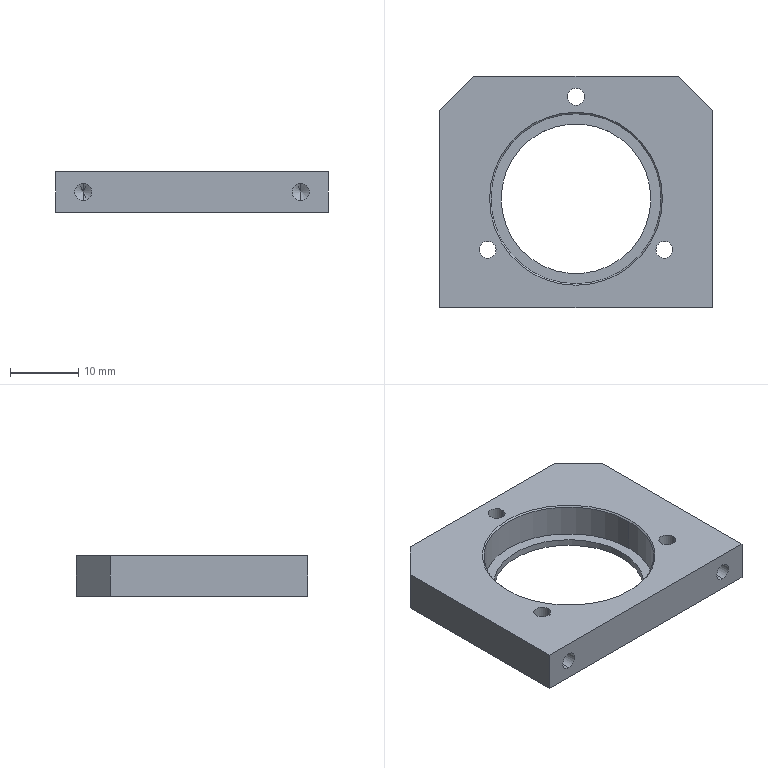Part | SolidWorks | features 3DProfileFeature 2, HoleWzd 2, Chamfer 1, Extrusion 1, ICE 1 | 1 solid | 29 faces | box 40 x 34 x 6 mm | volume 5024 mm3 | cylinder 14 | plane 9 | cone 6 | commonest cylinder face diameters 2.5 x10 22 x2 25 x2
STEP:
#1=CARTESIAN_POINT('',(-12.5,0.,5.8));
#2=VERTEX_POINT('',#1);
#3=CARTESIAN_POINT('',(12.5,0.,5.8));
#4=VERTEX_POINT('',#3);
#5=CARTESIAN_POINT('',(0.,0.,5.8));
#6=DIRECTION('',(0.,0.,1.));
#7=DIRECTION('',(1.,0.,0.));
#8=AXIS2_PLACEMENT_3D('',#5,#6,#7);
#9=CIRCLE('',#8,12.5);
#10=EDGE_CURVE('',#2,#4,#9,.T.);
#11=ORIENTED_EDGE('',*,*,#10,.F.);
#12=CARTESIAN_POINT('',(-12.7,0.,6.));
#13=VERTEX_POINT('',#12);
#14=CARTESIAN_POINT('',(-12.5,0.,5.8));
#15=DIRECTION('',(-0.7071,0.,0.7071));
#16=VECTOR('',#15,1000.);
#17=LINE('',#14,#16);
#18=EDGE_CURVE('',#2,#13,#17,.T.);
#19=ORIENTED_EDGE('',*,*,#18,.T.);
#20=CARTESIAN_POINT('',(12.7,0.,6.));
#21=VERTEX_POINT('',#20);
#22=CARTESIAN_POINT('',(0.,0.,6.));
#23=DIRECTION('',(0.,0.,-1.));
#24=DIRECTION('',(1.,0.,0.));
#25=AXIS2_PLACEMENT_3D('',#22,#23,#24);
#26=CIRCLE('',#25,12.7);
#27=EDGE_CURVE('',#21,#13,#26,.T.);
#28=ORIENTED_EDGE('',*,*,#27,.F.);
#29=CARTESIAN_POINT('',(12.5,0.,5.8));
#30=DIRECTION('',(0.7071,0.,0.7071));
#31=VECTOR('',#30,1000.);
#32=LINE('',#29,#31);
#33=EDGE_CURVE('',#4,#21,#32,.T.);
#34=ORIENTED_EDGE('',*,*,#33,.F.);
#35=EDGE_LOOP('',(#11,#19,#28,#34));
#36=FACE_OUTER_BOUND('',#35,.T.);
#37=CARTESIAN_POINT('',(0.,0.,5.8));
#38=DIRECTION('',(0.,0.,1.));
#39=DIRECTION('',(1.,0.,0.));
#40=AXIS2_PLACEMENT_3D('',#37,#38,#39);
#41=CONICAL_SURFACE('',#40,12.5,0.7854);
#42=ADVANCED_FACE('',(#36),#41,.F.);
#43=CARTESIAN_POINT('',(-16.,-10.,4.25));
#44=VERTEX_POINT('',#43);
#45=CARTESIAN_POINT('',(-16.,-10.,1.75));
#46=VERTEX_POINT('',#45);
#47=CARTESIAN_POINT('',(-16.,-10.,3.));
#48=DIRECTION('',(0.,-1.,0.));
#49=DIRECTION('',(0.,0.,-1.));
#50=AXIS2_PLACEMENT_3D('',#47,#48,#49);
#51=CIRCLE('',#50,1.25);
#52=EDGE_CURVE('',#44,#46,#51,.T.);
#53=ORIENTED_EDGE('',*,*,#52,.F.);
#54=CARTESIAN_POINT('',(-16.,-16.,4.25));
#55=VERTEX_POINT('',#54);
#56=CARTESIAN_POINT('',(-16.,-16.,4.25));
#57=DIRECTION('',(0.,-1.,0.));
#58=VECTOR('',#57,1000.);
#59=LINE('',#56,#58);
#60=EDGE_CURVE('',#44,#55,#59,.T.);
#61=ORIENTED_EDGE('',*,*,#60,.T.);
#62=CARTESIAN_POINT('',(-16.,-16.,1.75));
#63=VERTEX_POINT('',#62);
#64=CARTESIAN_POINT('',(-16.,-16.,3.));
#65=DIRECTION('',(0.,-1.,0.));
#66=DIRECTION('',(0.,0.,-1.));
#67=AXIS2_PLACEMENT_3D('',#64,#65,#66);
#68=CIRCLE('',#67,1.25);
#69=EDGE_CURVE('',#55,#63,#68,.T.);
#70=ORIENTED_EDGE('',*,*,#69,.T.);
#71=CARTESIAN_POINT('',(-16.,-16.,1.75));
#72=DIRECTION('',(0.,-1.,0.));
#73=VECTOR('',#72,1000.);
#74=LINE('',#71,#73);
#75=EDGE_CURVE('',#46,#63,#74,.T.);
#76=ORIENTED_EDGE('',*,*,#75,.F.);
#77=EDGE_LOOP('',(#53,#61,#70,#76));
#78=FACE_OUTER_BOUND('',#77,.T.);
#79=CARTESIAN_POINT('',(-16.,-16.,3.));
#80=DIRECTION('',(0.,-1.,0.));
#81=DIRECTION('',(0.,0.,-1.));
#82=AXIS2_PLACEMENT_3D('',#79,#80,#81);
#83=CYLINDRICAL_SURFACE('',#82,1.25);
#84=ADVANCED_FACE('',(#78),#83,.F.);
#85=CARTESIAN_POINT('',(-16.,-9.249,3.));
#86=VERTEX_POINT('',#85);
#87=CARTESIAN_POINT('',(-16.,-10.,1.75));
#88=DIRECTION('',(0.,-0.515,-0.8572));
#89=VECTOR('',#88,1000.);
#90=LINE('',#87,#89);
#91=EDGE_CURVE('',#86,#46,#90,.T.);
#92=ORIENTED_EDGE('',*,*,#91,.F.);
#93=CARTESIAN_POINT('',(-16.,-10.,4.25));
#94=DIRECTION('',(0.,-0.515,0.8572));
#95=VECTOR('',#94,1000.);
#96=LINE('',#93,#95);
#97=EDGE_CURVE('',#86,#44,#96,.T.);
#98=ORIENTED_EDGE('',*,*,#97,.T.);
#99=ORIENTED_EDGE('',*,*,#52,.T.);
#100=EDGE_LOOP('',(#92,#98,#99));
#101=FACE_OUTER_BOUND('',#100,.T.);
#102=CARTESIAN_POINT('',(-16.,-10.,3.));
#103=DIRECTION('',(0.,-1.,0.));
#104=DIRECTION('',(0.,0.,-1.));
#105=AXIS2_PLACEMENT_3D('',#102,#103,#104);
#106=CONICAL_SURFACE('',#105,1.25,1.03);
#107=ADVANCED_FACE('',(#101),#106,.F.);
#108=CARTESIAN_POINT('',(16.,-10.,4.25));
#109=VERTEX_POINT('',#108);
#110=CARTESIAN_POINT('',(16.,-10.,1.75));
#111=VERTEX_POINT('',#110);
#112=CARTESIAN_POINT('',(16.,-10.,3.));
#113=DIRECTION('',(0.,-1.,0.));
#114=DIRECTION('',(0.,0.,-1.));
#115=AXIS2_PLACEMENT_3D('',#112,#113,#114);
#116=CIRCLE('',#115,1.25);
#117=EDGE_CURVE('',#109,#111,#116,.T.);
#118=ORIENTED_EDGE('',*,*,#117,.F.);
#119=CARTESIAN_POINT('',(16.,-16.,4.25));
#120=VERTEX_POINT('',#119);
#121=CARTESIAN_POINT('',(16.,-16.,4.25));
#122=DIRECTION('',(0.,-1.,0.));
#123=VECTOR('',#122,1000.);
#124=LINE('',#121,#123);
#125=EDGE_CURVE('',#109,#120,#124,.T.);
#126=ORIENTED_EDGE('',*,*,#125,.T.);
#127=CARTESIAN_POINT('',(16.,-16.,1.75));
#128=VERTEX_POINT('',#127);
#129=CARTESIAN_POINT('',(16.,-16.,3.));
#130=DIRECTION('',(0.,-1.,0.));
#131=DIRECTION('',(0.,0.,-1.));
#132=AXIS2_PLACEMENT_3D('',#129,#130,#131);
#133=CIRCLE('',#132,1.25);
#134=EDGE_CURVE('',#120,#128,#133,.T.);
#135=ORIENTED_EDGE('',*,*,#134,.T.);
#136=CARTESIAN_POINT('',(16.,-16.,1.75));
#137=DIRECTION('',(0.,-1.,0.));
#138=VECTOR('',#137,1000.);
#139=LINE('',#136,#138);
#140=EDGE_CURVE('',#111,#128,#139,.T.);
#141=ORIENTED_EDGE('',*,*,#140,.F.);
#142=EDGE_LOOP('',(#118,#126,#135,#141));
#143=FACE_OUTER_BOUND('',#142,.T.);
#144=CARTESIAN_POINT('',(16.,-16.,3.));
#145=DIRECTION('',(0.,-1.,0.));
#146=DIRECTION('',(0.,0.,-1.));
#147=AXIS2_PLACEMENT_3D('',#144,#145,#146);
#148=CYLINDRICAL_SURFACE('',#147,1.25);
#149=ADVANCED_FACE('',(#143),#148,.F.);
#150=CARTESIAN_POINT('',(16.,-9.249,3.));
#151=VERTEX_POINT('',#150);
#152=CARTESIAN_POINT('',(16.,-10.,1.75));
#153=DIRECTION('',(0.,-0.515,-0.8572));
#154=VECTOR('',#153,1000.);
#155=LINE('',#152,#154);
#156=EDGE_CURVE('',#151,#111,#155,.T.);
#157=ORIENTED_EDGE('',*,*,#156,.F.);
#158=CARTESIAN_POINT('',(16.,-10.,4.25));
#159=DIRECTION('',(0.,-0.515,0.8572));
#160=VECTOR('',#159,1000.);
#161=LINE('',#158,#160);
#162=EDGE_CURVE('',#151,#109,#161,.T.);
#163=ORIENTED_EDGE('',*,*,#162,.T.);
#164=ORIENTED_EDGE('',*,*,#117,.T.);
#165=EDGE_LOOP('',(#157,#163,#164));
#166=FACE_OUTER_BOUND('',#165,.T.);
#167=CARTESIAN_POINT('',(16.,-10.,3.));
#168=DIRECTION('',(0.,-1.,0.));
#169=DIRECTION('',(0.,0.,-1.));
#170=AXIS2_PLACEMENT_3D('',#167,#168,#169);
#171=CONICAL_SURFACE('',#170,1.25,1.03);
#172=ADVANCED_FACE('',(#166),#171,.F.);
#173=CARTESIAN_POINT('',(-1.25,15.006,0.));
#174=VERTEX_POINT('',#173);
#175=CARTESIAN_POINT('',(1.25,15.006,0.));
#176=VERTEX_POINT('',#175);
#177=CARTESIAN_POINT('',(0.,15.006,0.));
#178=DIRECTION('',(0.,0.,1.));
#179=DIRECTION('',(1.,0.,0.));
#180=AXIS2_PLACEMENT_3D('',#177,#178,#179);
#181=CIRCLE('',#180,1.25);
#182=EDGE_CURVE('',#174,#176,#181,.T.);
#183=ORIENTED_EDGE('',*,*,#182,.F.);
#184=CARTESIAN_POINT('',(-1.25,15.006,6.));
#185=VERTEX_POINT('',#184);
#186=CARTESIAN_POINT('',(-1.25,15.006,6.));
#187=DIRECTION('',(0.,0.,1.));
#188=VECTOR('',#187,1000.);
#189=LINE('',#186,#188);
#190=EDGE_CURVE('',#174,#185,#189,.T.);
#191=ORIENTED_EDGE('',*,*,#190,.T.);
#192=CARTESIAN_POINT('',(1.25,15.006,6.));
#193=VERTEX_POINT('',#192);
#194=CARTESIAN_POINT('',(0.,15.006,6.));
#195=DIRECTION('',(0.,0.,1.));
#196=DIRECTION('',(1.,0.,0.));
#197=AXIS2_PLACEMENT_3D('',#194,#195,#196);
#198=CIRCLE('',#197,1.25);
#199=EDGE_CURVE('',#185,#193,#198,.T.);
#200=ORIENTED_EDGE('',*,*,#199,.T.);
#201=CARTESIAN_POINT('',(1.25,15.006,6.));
#202=DIRECTION('',(0.,0.,1.));
#203=VECTOR('',#202,1000.);
#204=LINE('',#201,#203);
#205=EDGE_CURVE('',#176,#193,#204,.T.);
#206=ORIENTED_EDGE('',*,*,#205,.F.);
#207=EDGE_LOOP('',(#183,#191,#200,#206));
#208=FACE_OUTER_BOUND('',#207,.T.);
#209=CARTESIAN_POINT('',(0.,15.006,6.));
#210=DIRECTION('',(0.,0.,1.));
#211=DIRECTION('',(1.,0.,0.));
#212=AXIS2_PLACEMENT_3D('',#209,#210,#211);
#213=CYLINDRICAL_SURFACE('',#212,1.25);
#214=ADVANCED_FACE('',(#208),#213,.F.);
#215=CARTESIAN_POINT('',(-14.24,-7.5,0.));
#216=VERTEX_POINT('',#215);
#217=CARTESIAN_POINT('',(-11.74,-7.5,0.));
#218=VERTEX_POINT('',#217);
#219=CARTESIAN_POINT('',(-12.99,-7.5,0.));
#220=DIRECTION('',(0.,0.,1.));
#221=DIRECTION('',(1.,0.,0.));
#222=AXIS2_PLACEMENT_3D('',#219,#220,#221);
#223=CIRCLE('',#222,1.25);
#224=EDGE_CURVE('',#216,#218,#223,.T.);
#225=ORIENTED_EDGE('',*,*,#224,.F.);
#226=CARTESIAN_POINT('',(-14.24,-7.5,6.));
#227=VERTEX_POINT('',#226);
#228=CARTESIAN_POINT('',(-14.24,-7.5,6.));
#229=DIRECTION('',(0.,0.,1.));
#230=VECTOR('',#229,1000.);
#231=LINE('',#228,#230);
#232=EDGE_CURVE('',#216,#227,#231,.T.);
#233=ORIENTED_EDGE('',*,*,#232,.T.);
#234=CARTESIAN_POINT('',(-11.74,-7.5,6.));
#235=VERTEX_POINT('',#234);
#236=CARTESIAN_POINT('',(-12.99,-7.5,6.));
#237=DIRECTION('',(0.,0.,1.));
#238=DIRECTION('',(1.,0.,0.));
#239=AXIS2_PLACEMENT_3D('',#236,#237,#238);
#240=CIRCLE('',#239,1.25);
#241=EDGE_CURVE('',#227,#235,#240,.T.);
#242=ORIENTED_EDGE('',*,*,#241,.T.);
#243=CARTESIAN_POINT('',(-11.74,-7.5,6.));
#244=DIRECTION('',(0.,0.,1.));
#245=VECTOR('',#244,1000.);
#246=LINE('',#243,#245);
#247=EDGE_CURVE('',#218,#235,#246,.T.);
#248=ORIENTED_EDGE('',*,*,#247,.F.);
#249=EDGE_LOOP('',(#225,#233,#242,#248));
#250=FACE_OUTER_BOUND('',#249,.T.);
#251=CARTESIAN_POINT('',(-12.99,-7.5,6.));
#252=DIRECTION('',(0.,0.,1.));
#253=DIRECTION('',(1.,0.,0.));
#254=AXIS2_PLACEMENT_3D('',#251,#252,#253);
#255=CYLINDRICAL_SURFACE('',#254,1.25);
#256=ADVANCED_FACE('',(#250),#255,.F.);
#257=CARTESIAN_POINT('',(11.74,-7.5,0.));
#258=VERTEX_POINT('',#257);
#259=CARTESIAN_POINT('',(14.24,-7.5,0.));
#260=VERTEX_POINT('',#259);
#261=CARTESIAN_POINT('',(12.99,-7.5,0.));
#262=DIRECTION('',(0.,0.,1.));
#263=DIRECTION('',(1.,0.,0.));
#264=AXIS2_PLACEMENT_3D('',#261,#262,#263);
#265=CIRCLE('',#264,1.25);
#266=EDGE_CURVE('',#258,#260,#265,.T.);
#267=ORIENTED_EDGE('',*,*,#266,.F.);
#268=CARTESIAN_POINT('',(11.74,-7.5,6.));
#269=VERTEX_POINT('',#268);
#270=CARTESIAN_POINT('',(11.74,-7.5,6.));
#271=DIRECTION('',(0.,0.,1.));
#272=VECTOR('',#271,1000.);
#273=LINE('',#270,#272);
#274=EDGE_CURVE('',#258,#269,#273,.T.);
#275=ORIENTED_EDGE('',*,*,#274,.T.);
#276=CARTESIAN_POINT('',(14.24,-7.5,6.));
#277=VERTEX_POINT('',#276);
#278=CARTESIAN_POINT('',(12.99,-7.5,6.));
#279=DIRECTION('',(0.,0.,1.));
#280=DIRECTION('',(1.,0.,0.));
#281=AXIS2_PLACEMENT_3D('',#278,#279,#280);
#282=CIRCLE('',#281,1.25);
#283=EDGE_CURVE('',#269,#277,#282,.T.);
#284=ORIENTED_EDGE('',*,*,#283,.T.);
#285=CARTESIAN_POINT('',(14.24,-7.5,6.));
#286=DIRECTION('',(0.,0.,1.));
#287=VECTOR('',#286,1000.);
#288=LINE('',#285,#287);
#289=EDGE_CURVE('',#260,#277,#288,.T.);
#290=ORIENTED_EDGE('',*,*,#289,.F.);
#291=EDGE_LOOP('',(#267,#275,#284,#290));
#292=FACE_OUTER_BOUND('',#291,.T.);
#293=CARTESIAN_POINT('',(12.99,-7.5,6.));
#294=DIRECTION('',(0.,0.,1.));
#295=DIRECTION('',(1.,0.,0.));
#296=AXIS2_PLACEMENT_3D('',#293,#294,#295);
#297=CYLINDRICAL_SURFACE('',#296,1.25);
#298=ADVANCED_FACE('',(#292),#297,.F.);
#299=CARTESIAN_POINT('',(-12.5,0.,1.));
#300=VERTEX_POINT('',#299);
#301=CARTESIAN_POINT('',(12.5,0.,1.));
#302=VERTEX_POINT('',#301);
#303=CARTESIAN_POINT('',(0.,0.,1.));
#304=DIRECTION('',(0.,0.,1.));
#305=DIRECTION('',(1.,0.,0.));
#306=AXIS2_PLACEMENT_3D('',#303,#304,#305);
#307=CIRCLE('',#306,12.5);
#308=EDGE_CURVE('',#300,#302,#307,.T.);
#309=ORIENTED_EDGE('',*,*,#308,.F.);
#310=CARTESIAN_POINT('',(-12.5,0.,1.));
#311=DIRECTION('',(0.,0.,1.));
#312=VECTOR('',#311,1000.);
#313=LINE('',#310,#312);
#314=EDGE_CURVE('',#300,#2,#313,.T.);
#315=ORIENTED_EDGE('',*,*,#314,.T.);
#316=ORIENTED_EDGE('',*,*,#10,.T.);
#317=CARTESIAN_POINT('',(12.5,0.,1.));
#318=DIRECTION('',(0.,0.,1.));
#319=VECTOR('',#318,1000.);
#320=LINE('',#317,#319);
#321=EDGE_CURVE('',#302,#4,#320,.T.);
#322=ORIENTED_EDGE('',*,*,#321,.F.);
#323=EDGE_LOOP('',(#309,#315,#316,#322));
#324=FACE_OUTER_BOUND('',#323,.T.);
#325=CARTESIAN_POINT('',(0.,0.,1.));
#326=DIRECTION('',(0.,0.,1.));
#327=DIRECTION('',(1.,0.,0.));
#328=AXIS2_PLACEMENT_3D('',#325,#326,#327);
#329=CYLINDRICAL_SURFACE('',#328,12.5);
#330=ADVANCED_FACE('',(#324),#329,.F.);
#331=CARTESIAN_POINT('',(-11.,0.,1.));
#332=VERTEX_POINT('',#331);
#333=CARTESIAN_POINT('',(11.,0.,1.));
#334=VERTEX_POINT('',#333);
#335=CARTESIAN_POINT('',(0.,0.,1.));
#336=DIRECTION('',(0.,0.,1.));
#337=DIRECTION('',(1.,0.,0.));
#338=AXIS2_PLACEMENT_3D('',#335,#336,#337);
#339=CIRCLE('',#338,11.);
#340=EDGE_CURVE('',#332,#334,#339,.T.);
#341=ORIENTED_EDGE('',*,*,#340,.T.);
#342=CARTESIAN_POINT('',(11.,0.,0.));
#343=VERTEX_POINT('',#342);
#344=CARTESIAN_POINT('',(11.,0.,6.));
#345=DIRECTION('',(0.,0.,-1.));
#346=VECTOR('',#345,1000.);
#347=LINE('',#344,#346);
#348=EDGE_CURVE('',#334,#343,#347,.T.);
#349=ORIENTED_EDGE('',*,*,#348,.T.);
#350=CARTESIAN_POINT('',(-11.,0.,0.));
#351=VERTEX_POINT('',#350);
#352=CARTESIAN_POINT('',(0.,0.,0.));
#353=DIRECTION('',(0.,0.,1.));
#354=DIRECTION('',(1.,0.,0.));
#355=AXIS2_PLACEMENT_3D('',#352,#353,#354);
#356=CIRCLE('',#355,11.);
#357=EDGE_CURVE('',#351,#343,#356,.T.);
#358=ORIENTED_EDGE('',*,*,#357,.F.);
#359=CARTESIAN_POINT('',(-11.,0.,6.));
#360=DIRECTION('',(0.,0.,-1.));
#361=VECTOR('',#360,1000.);
#362=LINE('',#359,#361);
#363=EDGE_CURVE('',#332,#351,#362,.T.);
#364=ORIENTED_EDGE('',*,*,#363,.F.);
#365=EDGE_LOOP('',(#341,#349,#358,#364));
#366=FACE_OUTER_BOUND('',#365,.T.);
#367=CARTESIAN_POINT('',(0.,0.,6.));
#368=DIRECTION('',(0.,0.,-1.));
#369=DIRECTION('',(-1.,0.,0.));
#370=AXIS2_PLACEMENT_3D('',#367,#368,#369);
#371=CYLINDRICAL_SURFACE('',#370,11.);
#372=ADVANCED_FACE('',(#366),#371,.F.);
#373=ORIENTED_EDGE('',*,*,#348,.F.);
#374=CARTESIAN_POINT('',(0.,0.,1.));
#375=DIRECTION('',(0.,0.,1.));
#376=DIRECTION('',(1.,0.,0.));
#377=AXIS2_PLACEMENT_3D('',#374,#375,#376);
#378=CIRCLE('',#377,11.);
#379=EDGE_CURVE('',#334,#332,#378,.T.);
#380=ORIENTED_EDGE('',*,*,#379,.T.);
#381=ORIENTED_EDGE('',*,*,#363,.T.);
#382=CARTESIAN_POINT('',(0.,0.,0.));
#383=DIRECTION('',(0.,0.,1.));
#384=DIRECTION('',(1.,0.,0.));
#385=AXIS2_PLACEMENT_3D('',#382,#383,#384);
#386=CIRCLE('',#385,11.);
#387=EDGE_CURVE('',#343,#351,#386,.T.);
#388=ORIENTED_EDGE('',*,*,#387,.F.);
#389=EDGE_LOOP('',(#373,#380,#381,#388));
#390=FACE_OUTER_BOUND('',#389,.T.);
#391=CARTESIAN_POINT('',(0.,0.,6.));
#392=DIRECTION('',(0.,0.,-1.));
#393=DIRECTION('',(-1.,0.,0.));
#394=AXIS2_PLACEMENT_3D('',#391,#392,#393);
#395=CYLINDRICAL_SURFACE('',#394,11.);
#396=ADVANCED_FACE('',(#390),#395,.F.);
#397=ORIENTED_EDGE('',*,*,#27,.T.);
#398=CARTESIAN_POINT('',(0.,0.,6.));
#399=DIRECTION('',(0.,0.,-1.));
#400=DIRECTION('',(1.,0.,0.));
#401=AXIS2_PLACEMENT_3D('',#398,#399,#400);
#402=CIRCLE('',#401,12.7);
#403=EDGE_CURVE('',#13,#21,#402,.T.);
#404=ORIENTED_EDGE('',*,*,#403,.T.);
#405=EDGE_LOOP('',(#397,#404));
#406=FACE_BOUND('',#405,.T.);
#407=CARTESIAN_POINT('',(0.,15.006,6.));
#408=DIRECTION('',(0.,0.,1.));
#409=DIRECTION('',(1.,0.,0.));
#410=AXIS2_PLACEMENT_3D('',#407,#408,#409);
#411=CIRCLE('',#410,1.25);
#412=EDGE_CURVE('',#193,#185,#411,.T.);
#413=ORIENTED_EDGE('',*,*,#412,.F.);
#414=ORIENTED_EDGE('',*,*,#199,.F.);
#415=EDGE_LOOP('',(#413,#414));
#416=FACE_BOUND('',#415,.T.);
#417=CARTESIAN_POINT('',(-12.99,-7.5,6.));
#418=DIRECTION('',(0.,0.,1.));
#419=DIRECTION('',(1.,0.,0.));
#420=AXIS2_PLACEMENT_3D('',#417,#418,#419);
#421=CIRCLE('',#420,1.25);
#422=EDGE_CURVE('',#235,#227,#421,.T.);
#423=ORIENTED_EDGE('',*,*,#422,.F.);
#424=ORIENTED_EDGE('',*,*,#241,.F.);
#425=EDGE_LOOP('',(#423,#424));
#426=FACE_BOUND('',#425,.T.);
#427=CARTESIAN_POINT('',(12.99,-7.5,6.));
#428=DIRECTION('',(0.,0.,1.));
#429=DIRECTION('',(1.,0.,0.));
#430=AXIS2_PLACEMENT_3D('',#427,#428,#429);
#431=CIRCLE('',#430,1.25);
#432=EDGE_CURVE('',#277,#269,#431,.T.);
#433=ORIENTED_EDGE('',*,*,#432,.F.);
#434=ORIENTED_EDGE('',*,*,#283,.F.);
#435=EDGE_LOOP('',(#433,#434));
#436=FACE_BOUND('',#435,.T.);
#437=CARTESIAN_POINT('',(20.,-16.,6.));
#438=VERTEX_POINT('',#437);
#439=CARTESIAN_POINT('',(20.,13.,6.));
#440=VERTEX_POINT('',#439);
#441=CARTESIAN_POINT('',(20.,13.,6.));
#442=DIRECTION('',(0.,1.,0.));
#443=VECTOR('',#442,1000.);
#444=LINE('',#441,#443);
#445=EDGE_CURVE('',#438,#440,#444,.T.);
#446=ORIENTED_EDGE('',*,*,#445,.T.);
#447=CARTESIAN_POINT('',(15.,18.,6.));
#448=VERTEX_POINT('',#447);
#449=CARTESIAN_POINT('',(15.,18.,6.));
#450=DIRECTION('',(-0.7071,0.7071,0.));
#451=VECTOR('',#450,1000.);
#452=LINE('',#449,#451);
#453=EDGE_CURVE('',#440,#448,#452,.T.);
#454=ORIENTED_EDGE('',*,*,#453,.T.);
#455=CARTESIAN_POINT('',(-15.,18.,6.));
#456=VERTEX_POINT('',#455);
#457=CARTESIAN_POINT('',(-15.,18.,6.));
#458=DIRECTION('',(-1.,0.,0.));
#459=VECTOR('',#458,1000.);
#460=LINE('',#457,#459);
#461=EDGE_CURVE('',#448,#456,#460,.T.);
#462=ORIENTED_EDGE('',*,*,#461,.T.);
#463=CARTESIAN_POINT('',(-20.,13.,6.));
#464=VERTEX_POINT('',#463);
#465=CARTESIAN_POINT('',(-20.,13.,6.));
#466=DIRECTION('',(-0.7071,-0.7071,0.));
#467=VECTOR('',#466,1000.);
#468=LINE('',#465,#467);
#469=EDGE_CURVE('',#456,#464,#468,.T.);
#470=ORIENTED_EDGE('',*,*,#469,.T.);
#471=CARTESIAN_POINT('',(-20.,-16.,6.));
#472=VERTEX_POINT('',#471);
#473=CARTESIAN_POINT('',(-20.,13.,6.));
#474=DIRECTION('',(0.,-1.,0.));
#475=VECTOR('',#474,1000.);
#476=LINE('',#473,#475);
#477=EDGE_CURVE('',#464,#472,#476,.T.);
#478=ORIENTED_EDGE('',*,*,#477,.T.);
#479=CARTESIAN_POINT('',(-20.,-16.,6.));
#480=DIRECTION('',(1.,0.,0.));
#481=VECTOR('',#480,1000.);
#482=LINE('',#479,#481);
#483=EDGE_CURVE('',#472,#438,#482,.T.);
#484=ORIENTED_EDGE('',*,*,#483,.T.);
#485=EDGE_LOOP('',(#446,#454,#462,#470,#478,#484));
#486=FACE_OUTER_BOUND('',#485,.T.);
#487=CARTESIAN_POINT('',(20.,-16.,6.));
#488=DIRECTION('',(0.,0.,1.));
#489=DIRECTION('',(1.,0.,0.));
#490=AXIS2_PLACEMENT_3D('',#487,#488,#489);
#491=PLANE('',#490);
#492=ADVANCED_FACE('',(#406,#416,#426,#436,#486),#491,.T.);
#493=CARTESIAN_POINT('',(0.,15.006,0.));
#494=DIRECTION('',(0.,0.,1.));
#495=DIRECTION('',(1.,0.,0.));
#496=AXIS2_PLACEMENT_3D('',#493,#494,#495);
#497=CIRCLE('',#496,1.25);
#498=EDGE_CURVE('',#176,#174,#497,.T.);
#499=ORIENTED_EDGE('',*,*,#498,.T.);
#500=ORIENTED_EDGE('',*,*,#182,.T.);
#501=EDGE_LOOP('',(#499,#500));
#502=FACE_BOUND('',#501,.T.);
#503=CARTESIAN_POINT('',(-12.99,-7.5,0.));
#504=DIRECTION('',(0.,0.,1.));
#505=DIRECTION('',(1.,0.,0.));
#506=AXIS2_PLACEMENT_3D('',#503,#504,#505);
#507=CIRCLE('',#506,1.25);
#508=EDGE_CURVE('',#218,#216,#507,.T.);
#509=ORIENTED_EDGE('',*,*,#508,.T.);
#510=ORIENTED_EDGE('',*,*,#224,.T.);
#511=EDGE_LOOP('',(#509,#510));
#512=FACE_BOUND('',#511,.T.);
#513=CARTESIAN_POINT('',(12.99,-7.5,0.));
#514=DIRECTION('',(0.,0.,1.));
#515=DIRECTION('',(1.,0.,0.));
#516=AXIS2_PLACEMENT_3D('',#513,#514,#515);
#517=CIRCLE('',#516,1.25);
#518=EDGE_CURVE('',#260,#258,#517,.T.);
#519=ORIENTED_EDGE('',*,*,#518,.T.);
#520=ORIENTED_EDGE('',*,*,#266,.T.);
#521=EDGE_LOOP('',(#519,#520));
#522=FACE_BOUND('',#521,.T.);
#523=CARTESIAN_POINT('',(20.,-16.,0.));
#524=VERTEX_POINT('',#523);
#525=CARTESIAN_POINT('',(20.,13.,0.));
#526=VERTEX_POINT('',#525);
#527=CARTESIAN_POINT('',(20.,13.,0.));
#528=DIRECTION('',(0.,1.,0.));
#529=VECTOR('',#528,1000.);
#530=LINE('',#527,#529);
#531=EDGE_CURVE('',#524,#526,#530,.T.);
#532=ORIENTED_EDGE('',*,*,#531,.F.);
#533=CARTESIAN_POINT('',(-20.,-16.,0.));
#534=VERTEX_POINT('',#533);
#535=CARTESIAN_POINT('',(-20.,-16.,0.));
#536=DIRECTION('',(1.,0.,0.));
#537=VECTOR('',#536,1000.);
#538=LINE('',#535,#537);
#539=EDGE_CURVE('',#534,#524,#538,.T.);
#540=ORIENTED_EDGE('',*,*,#539,.F.);
#541=CARTESIAN_POINT('',(-20.,13.,0.));
#542=VERTEX_POINT('',#541);
#543=CARTESIAN_POINT('',(-20.,13.,0.));
#544=DIRECTION('',(0.,-1.,0.));
#545=VECTOR('',#544,1000.);
#546=LINE('',#543,#545);
#547=EDGE_CURVE('',#542,#534,#546,.T.);
#548=ORIENTED_EDGE('',*,*,#547,.F.);
#549=CARTESIAN_POINT('',(-15.,18.,0.));
#550=VERTEX_POINT('',#549);
#551=CARTESIAN_POINT('',(-20.,13.,0.));
#552=DIRECTION('',(-0.7071,-0.7071,0.));
#553=VECTOR('',#552,1000.);
#554=LINE('',#551,#553);
#555=EDGE_CURVE('',#550,#542,#554,.T.);
#556=ORIENTED_EDGE('',*,*,#555,.F.);
#557=CARTESIAN_POINT('',(15.,18.,0.));
#558=VERTEX_POINT('',#557);
#559=CARTESIAN_POINT('',(-15.,18.,0.));
#560=DIRECTION('',(-1.,0.,0.));
#561=VECTOR('',#560,1000.);
#562=LINE('',#559,#561);
#563=EDGE_CURVE('',#558,#550,#562,.T.);
#564=ORIENTED_EDGE('',*,*,#563,.F.);
#565=CARTESIAN_POINT('',(15.,18.,0.));
#566=DIRECTION('',(-0.7071,0.7071,0.));
#567=VECTOR('',#566,1000.);
#568=LINE('',#565,#567);
#569=EDGE_CURVE('',#526,#558,#568,.T.);
#570=ORIENTED_EDGE('',*,*,#569,.F.);
#571=EDGE_LOOP('',(#532,#540,#548,#556,#564,#570));
#572=FACE_OUTER_BOUND('',#571,.T.);
#573=ORIENTED_EDGE('',*,*,#357,.T.);
#574=ORIENTED_EDGE('',*,*,#387,.T.);
#575=EDGE_LOOP('',(#573,#574));
#576=FACE_BOUND('',#575,.T.);
#577=CARTESIAN_POINT('',(20.,-16.,0.));
#578=DIRECTION('',(0.,0.,1.));
#579=DIRECTION('',(1.,0.,0.));
#580=AXIS2_PLACEMENT_3D('',#577,#578,#579);
#581=PLANE('',#580);
#582=ADVANCED_FACE('',(#502,#512,#522,#572,#576),#581,.F.);
#583=ORIENTED_EDGE('',*,*,#531,.T.);
#584=CARTESIAN_POINT('',(20.,13.,6.));
#585=DIRECTION('',(0.,0.,-1.));
#586=VECTOR('',#585,1000.);
#587=LINE('',#584,#586);
#588=EDGE_CURVE('',#440,#526,#587,.T.);
#589=ORIENTED_EDGE('',*,*,#588,.F.);
#590=ORIENTED_EDGE('',*,*,#445,.F.);
#591=CARTESIAN_POINT('',(20.,-16.,6.));
#592=DIRECTION('',(0.,0.,-1.));
#593=VECTOR('',#592,1000.);
#594=LINE('',#591,#593);
#595=EDGE_CURVE('',#438,#524,#594,.T.);
#596=ORIENTED_EDGE('',*,*,#595,.T.);
#597=EDGE_LOOP('',(#583,#589,#590,#596));
#598=FACE_OUTER_BOUND('',#597,.T.);
#599=CARTESIAN_POINT('',(20.,13.,6.));
#600=DIRECTION('',(-1.,0.,0.));
#601=DIRECTION('',(0.,-1.,0.));
#602=AXIS2_PLACEMENT_3D('',#599,#600,#601);
#603=PLANE('',#602);
#604=ADVANCED_FACE('',(#598),#603,.F.);
#605=ORIENTED_EDGE('',*,*,#569,.T.);
#606=CARTESIAN_POINT('',(15.,18.,6.));
#607=DIRECTION('',(0.,0.,-1.));
#608=VECTOR('',#607,1000.);
#609=LINE('',#606,#608);
#610=EDGE_CURVE('',#448,#558,#609,.T.);
#611=ORIENTED_EDGE('',*,*,#610,.F.);
#612=ORIENTED_EDGE('',*,*,#453,.F.);
#613=ORIENTED_EDGE('',*,*,#588,.T.);
#614=EDGE_LOOP('',(#605,#611,#612,#613));
#615=FACE_OUTER_BOUND('',#614,.T.);
#616=CARTESIAN_POINT('',(15.,18.,6.));
#617=DIRECTION('',(-0.7071,-0.7071,0.));
#618=DIRECTION('',(0.7071,-0.7071,0.));
#619=AXIS2_PLACEMENT_3D('',#616,#617,#618);
#620=PLANE('',#619);
#621=ADVANCED_FACE('',(#615),#620,.F.);
#622=ORIENTED_EDGE('',*,*,#563,.T.);
#623=CARTESIAN_POINT('',(-15.,18.,6.));
#624=DIRECTION('',(0.,0.,-1.));
#625=VECTOR('',#624,1000.);
#626=LINE('',#623,#625);
#627=EDGE_CURVE('',#456,#550,#626,.T.);
#628=ORIENTED_EDGE('',*,*,#627,.F.);
#629=ORIENTED_EDGE('',*,*,#461,.F.);
#630=ORIENTED_EDGE('',*,*,#610,.T.);
#631=EDGE_LOOP('',(#622,#628,#629,#630));
#632=FACE_OUTER_BOUND('',#631,.T.);
#633=CARTESIAN_POINT('',(-15.,18.,6.));
#634=DIRECTION('',(0.,-1.,0.));
#635=DIRECTION('',(0.,0.,-1.));
#636=AXIS2_PLACEMENT_3D('',#633,#634,#635);
#637=PLANE('',#636);
#638=ADVANCED_FACE('',(#632),#637,.F.);
#639=ORIENTED_EDGE('',*,*,#555,.T.);
#640=CARTESIAN_POINT('',(-20.,13.,6.));
#641=DIRECTION('',(0.,0.,-1.));
#642=VECTOR('',#641,1000.);
#643=LINE('',#640,#642);
#644=EDGE_CURVE('',#464,#542,#643,.T.);
#645=ORIENTED_EDGE('',*,*,#644,.F.);
#646=ORIENTED_EDGE('',*,*,#469,.F.);
#647=ORIENTED_EDGE('',*,*,#627,.T.);
#648=EDGE_LOOP('',(#639,#645,#646,#647));
#649=FACE_OUTER_BOUND('',#648,.T.);
#650=CARTESIAN_POINT('',(-20.,13.,6.));
#651=DIRECTION('',(0.7071,-0.7071,0.));
#652=DIRECTION('',(0.7071,0.7071,0.));
#653=AXIS2_PLACEMENT_3D('',#650,#651,#652);
#654=PLANE('',#653);
#655=ADVANCED_FACE('',(#649),#654,.F.);
#656=ORIENTED_EDGE('',*,*,#547,.T.);
#657=CARTESIAN_POINT('',(-20.,-16.,6.));
#658=DIRECTION('',(0.,0.,-1.));
#659=VECTOR('',#658,1000.);
#660=LINE('',#657,#659);
#661=EDGE_CURVE('',#472,#534,#660,.T.);
#662=ORIENTED_EDGE('',*,*,#661,.F.);
#663=ORIENTED_EDGE('',*,*,#477,.F.);
#664=ORIENTED_EDGE('',*,*,#644,.T.);
#665=EDGE_LOOP('',(#656,#662,#663,#664));
#666=FACE_OUTER_BOUND('',#665,.T.);
#667=CARTESIAN_POINT('',(-20.,13.,6.));
#668=DIRECTION('',(1.,0.,0.));
#669=DIRECTION('',(0.,0.,-1.));
#670=AXIS2_PLACEMENT_3D('',#667,#668,#669);
#671=PLANE('',#670);
#672=ADVANCED_FACE('',(#666),#671,.F.);
#673=CARTESIAN_POINT('',(-16.,-16.,3.));
#674=DIRECTION('',(0.,-1.,0.));
#675=DIRECTION('',(0.,0.,-1.));
#676=AXIS2_PLACEMENT_3D('',#673,#674,#675);
#677=CIRCLE('',#676,1.25);
#678=EDGE_CURVE('',#63,#55,#677,.T.);
#679=ORIENTED_EDGE('',*,*,#678,.F.);
#680=ORIENTED_EDGE('',*,*,#69,.F.);
#681=EDGE_LOOP('',(#679,#680));
#682=FACE_BOUND('',#681,.T.);
#683=CARTESIAN_POINT('',(16.,-16.,3.));
#684=DIRECTION('',(0.,-1.,0.));
#685=DIRECTION('',(0.,0.,-1.));
#686=AXIS2_PLACEMENT_3D('',#683,#684,#685);
#687=CIRCLE('',#686,1.25);
#688=EDGE_CURVE('',#128,#120,#687,.T.);
#689=ORIENTED_EDGE('',*,*,#688,.F.);
#690=ORIENTED_EDGE('',*,*,#134,.F.);
#691=EDGE_LOOP('',(#689,#690));
#692=FACE_BOUND('',#691,.T.);
#693=ORIENTED_EDGE('',*,*,#539,.T.);
#694=ORIENTED_EDGE('',*,*,#595,.F.);
#695=ORIENTED_EDGE('',*,*,#483,.F.);
#696=ORIENTED_EDGE('',*,*,#661,.T.);
#697=EDGE_LOOP('',(#693,#694,#695,#696));
#698=FACE_OUTER_BOUND('',#697,.T.);
#699=CARTESIAN_POINT('',(-20.,-16.,6.));
#700=DIRECTION('',(0.,1.,0.));
#701=DIRECTION('',(0.,0.,1.));
#702=AXIS2_PLACEMENT_3D('',#699,#700,#701);
#703=PLANE('',#702);
#704=ADVANCED_FACE('',(#682,#692,#698),#703,.F.);
#705=ORIENTED_EDGE('',*,*,#314,.F.);
#706=CARTESIAN_POINT('',(0.,0.,1.));
#707=DIRECTION('',(0.,0.,1.));
#708=DIRECTION('',(1.,0.,0.));
#709=AXIS2_PLACEMENT_3D('',#706,#707,#708);
#710=CIRCLE('',#709,12.5);
#711=EDGE_CURVE('',#302,#300,#710,.T.);
#712=ORIENTED_EDGE('',*,*,#711,.F.);
#713=ORIENTED_EDGE('',*,*,#321,.T.);
#714=CARTESIAN_POINT('',(0.,0.,5.8));
#715=DIRECTION('',(0.,0.,1.));
#716=DIRECTION('',(1.,0.,0.));
#717=AXIS2_PLACEMENT_3D('',#714,#715,#716);
#718=CIRCLE('',#717,12.5);
#719=EDGE_CURVE('',#4,#2,#718,.T.);
#720=ORIENTED_EDGE('',*,*,#719,.T.);
#721=EDGE_LOOP('',(#705,#712,#713,#720));
#722=FACE_OUTER_BOUND('',#721,.T.);
#723=CARTESIAN_POINT('',(0.,0.,1.));
#724=DIRECTION('',(0.,0.,1.));
#725=DIRECTION('',(1.,0.,0.));
#726=AXIS2_PLACEMENT_3D('',#723,#724,#725);
#727=CYLINDRICAL_SURFACE('',#726,12.5);
#728=ADVANCED_FACE('',(#722),#727,.F.);
#729=ORIENTED_EDGE('',*,*,#340,.F.);
#730=ORIENTED_EDGE('',*,*,#379,.F.);
#731=EDGE_LOOP('',(#729,#730));
#732=FACE_BOUND('',#731,.T.);
#733=ORIENTED_EDGE('',*,*,#711,.T.);
#734=ORIENTED_EDGE('',*,*,#308,.T.);
#735=EDGE_LOOP('',(#733,#734));
#736=FACE_OUTER_BOUND('',#735,.T.);
#737=CARTESIAN_POINT('',(0.,0.,1.));
#738=DIRECTION('',(0.,0.,1.));
#739=DIRECTION('',(1.,0.,0.));
#740=AXIS2_PLACEMENT_3D('',#737,#738,#739);
#741=PLANE('',#740);
#742=ADVANCED_FACE('',(#732,#736),#741,.T.);
#743=ORIENTED_EDGE('',*,*,#274,.F.);
#744=ORIENTED_EDGE('',*,*,#518,.F.);
#745=ORIENTED_EDGE('',*,*,#289,.T.);
#746=ORIENTED_EDGE('',*,*,#432,.T.);
#747=EDGE_LOOP('',(#743,#744,#745,#746));
#748=FACE_OUTER_BOUND('',#747,.T.);
#749=CARTESIAN_POINT('',(12.99,-7.5,6.));
#750=DIRECTION('',(0.,0.,1.));
#751=DIRECTION('',(1.,0.,0.));
#752=AXIS2_PLACEMENT_3D('',#749,#750,#751);
#753=CYLINDRICAL_SURFACE('',#752,1.25);
#754=ADVANCED_FACE('',(#748),#753,.F.);
#755=ORIENTED_EDGE('',*,*,#232,.F.);
#756=ORIENTED_EDGE('',*,*,#508,.F.);
#757=ORIENTED_EDGE('',*,*,#247,.T.);
#758=ORIENTED_EDGE('',*,*,#422,.T.);
#759=EDGE_LOOP('',(#755,#756,#757,#758));
#760=FACE_OUTER_BOUND('',#759,.T.);
#761=CARTESIAN_POINT('',(-12.99,-7.5,6.));
#762=DIRECTION('',(0.,0.,1.));
#763=DIRECTION('',(1.,0.,0.));
#764=AXIS2_PLACEMENT_3D('',#761,#762,#763);
#765=CYLINDRICAL_SURFACE('',#764,1.25);
#766=ADVANCED_FACE('',(#760),#765,.F.);
#767=ORIENTED_EDGE('',*,*,#190,.F.);
#768=ORIENTED_EDGE('',*,*,#498,.F.);
#769=ORIENTED_EDGE('',*,*,#205,.T.);
#770=ORIENTED_EDGE('',*,*,#412,.T.);
#771=EDGE_LOOP('',(#767,#768,#769,#770));
#772=FACE_OUTER_BOUND('',#771,.T.);
#773=CARTESIAN_POINT('',(0.,15.006,6.));
#774=DIRECTION('',(0.,0.,1.));
#775=DIRECTION('',(1.,0.,0.));
#776=AXIS2_PLACEMENT_3D('',#773,#774,#775);
#777=CYLINDRICAL_SURFACE('',#776,1.25);
#778=ADVANCED_FACE('',(#772),#777,.F.);
#779=ORIENTED_EDGE('',*,*,#162,.F.);
#780=ORIENTED_EDGE('',*,*,#156,.T.);
#781=CARTESIAN_POINT('',(16.,-10.,3.));
#782=DIRECTION('',(0.,-1.,0.));
#783=DIRECTION('',(0.,0.,-1.));
#784=AXIS2_PLACEMENT_3D('',#781,#782,#783);
#785=CIRCLE('',#784,1.25);
#786=EDGE_CURVE('',#111,#109,#785,.T.);
#787=ORIENTED_EDGE('',*,*,#786,.T.);
#788=EDGE_LOOP('',(#779,#780,#787));
#789=FACE_OUTER_BOUND('',#788,.T.);
#790=CARTESIAN_POINT('',(16.,-10.,3.));
#791=DIRECTION('',(0.,-1.,0.));
#792=DIRECTION('',(0.,0.,-1.));
#793=AXIS2_PLACEMENT_3D('',#790,#791,#792);
#794=CONICAL_SURFACE('',#793,1.25,1.03);
#795=ADVANCED_FACE('',(#789),#794,.F.);
#796=ORIENTED_EDGE('',*,*,#125,.F.);
#797=ORIENTED_EDGE('',*,*,#786,.F.);
#798=ORIENTED_EDGE('',*,*,#140,.T.);
#799=ORIENTED_EDGE('',*,*,#688,.T.);
#800=EDGE_LOOP('',(#796,#797,#798,#799));
#801=FACE_OUTER_BOUND('',#800,.T.);
#802=CARTESIAN_POINT('',(16.,-16.,3.));
#803=DIRECTION('',(0.,-1.,0.));
#804=DIRECTION('',(0.,0.,-1.));
#805=AXIS2_PLACEMENT_3D('',#802,#803,#804);
#806=CYLINDRICAL_SURFACE('',#805,1.25);
#807=ADVANCED_FACE('',(#801),#806,.F.);
#808=ORIENTED_EDGE('',*,*,#97,.F.);
#809=ORIENTED_EDGE('',*,*,#91,.T.);
#810=CARTESIAN_POINT('',(-16.,-10.,3.));
#811=DIRECTION('',(0.,-1.,0.));
#812=DIRECTION('',(0.,0.,-1.));
#813=AXIS2_PLACEMENT_3D('',#810,#811,#812);
#814=CIRCLE('',#813,1.25);
#815=EDGE_CURVE('',#46,#44,#814,.T.);
#816=ORIENTED_EDGE('',*,*,#815,.T.);
#817=EDGE_LOOP('',(#808,#809,#816));
#818=FACE_OUTER_BOUND('',#817,.T.);
#819=CARTESIAN_POINT('',(-16.,-10.,3.));
#820=DIRECTION('',(0.,-1.,0.));
#821=DIRECTION('',(0.,0.,-1.));
#822=AXIS2_PLACEMENT_3D('',#819,#820,#821);
#823=CONICAL_SURFACE('',#822,1.25,1.03);
#824=ADVANCED_FACE('',(#818),#823,.F.);
#825=ORIENTED_EDGE('',*,*,#60,.F.);
#826=ORIENTED_EDGE('',*,*,#815,.F.);
#827=ORIENTED_EDGE('',*,*,#75,.T.);
#828=ORIENTED_EDGE('',*,*,#678,.T.);
#829=EDGE_LOOP('',(#825,#826,#827,#828));
#830=FACE_OUTER_BOUND('',#829,.T.);
#831=CARTESIAN_POINT('',(-16.,-16.,3.));
#832=DIRECTION('',(0.,-1.,0.));
#833=DIRECTION('',(0.,0.,-1.));
#834=AXIS2_PLACEMENT_3D('',#831,#832,#833);
#835=CYLINDRICAL_SURFACE('',#834,1.25);
#836=ADVANCED_FACE('',(#830),#835,.F.);
#837=ORIENTED_EDGE('',*,*,#18,.F.);
#838=ORIENTED_EDGE('',*,*,#719,.F.);
#839=ORIENTED_EDGE('',*,*,#33,.T.);
#840=ORIENTED_EDGE('',*,*,#403,.F.);
#841=EDGE_LOOP('',(#837,#838,#839,#840));
#842=FACE_OUTER_BOUND('',#841,.T.);
#843=CARTESIAN_POINT('',(0.,0.,5.8));
#844=DIRECTION('',(0.,0.,1.));
#845=DIRECTION('',(1.,0.,0.));
#846=AXIS2_PLACEMENT_3D('',#843,#844,#845);
#847=CONICAL_SURFACE('',#846,12.5,0.7854);
#848=ADVANCED_FACE('',(#842),#847,.F.);
#849=CLOSED_SHELL('',(#42,#84,#107,#149,#172,#214,#256,#298,#330,#372,#396,#492,#582,#604,#621,#638,#655,#672,#704,#728,#742,#754,#766,#778,#795,#807,#824,#836,#848));
#850=MANIFOLD_SOLID_BREP('',#849);
#851=CARTESIAN_POINT('',(0.,0.,0.));
#852=DIRECTION('',(0.,0.,1.));
#853=DIRECTION('',(1.,0.,0.));
#854=AXIS2_PLACEMENT_3D('',#851,#852,#853);
#855=(LENGTH_UNIT()NAMED_UNIT(*)SI_UNIT(.MILLI.,.METRE.));
#856=UNCERTAINTY_MEASURE_WITH_UNIT(LENGTH_MEASURE(0.00001),#855,'','');
#857=(NAMED_UNIT(*)PLANE_ANGLE_UNIT()SI_UNIT($,.RADIAN.));
#858=(NAMED_UNIT(*)SI_UNIT($,.STERADIAN.)SOLID_ANGLE_UNIT());
#859=(GEOMETRIC_REPRESENTATION_CONTEXT(3)GLOBAL_UNCERTAINTY_ASSIGNED_CONTEXT((#856))GLOBAL_UNIT_ASSIGNED_CONTEXT((#855,#857,#858))REPRESENTATION_CONTEXT('',''));
#860=ADVANCED_BREP_SHAPE_REPRESENTATION('',(#850,#854),#859);